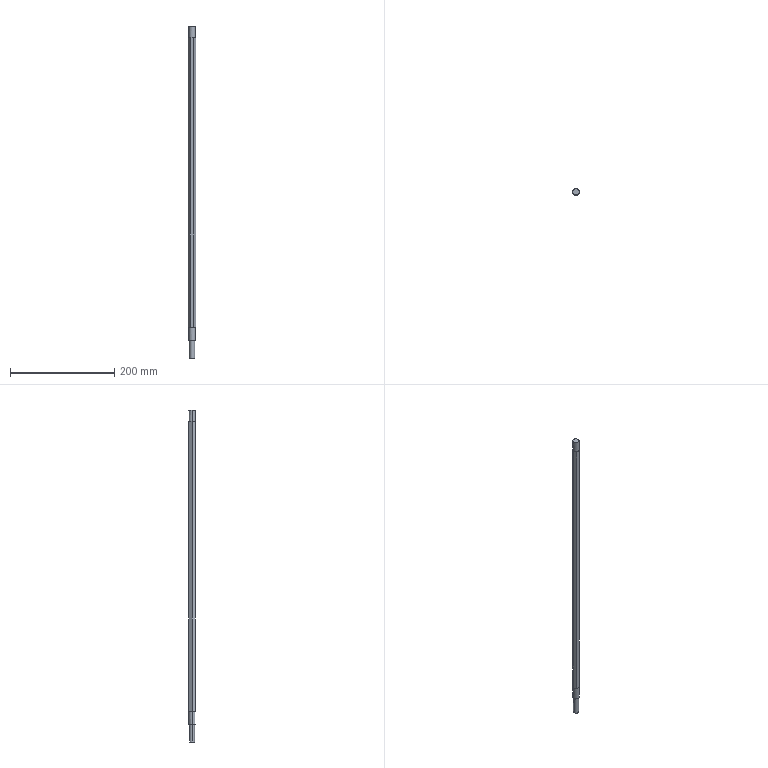Part | SolidWorks | features BaseBody 1 | 1 solid | 31 faces | box 13.856 x 12 x 637 mm | volume 77091 mm3 | plane 24 | cylinder 7 | commonest cylinder face diameters 12 x4 10 x2 3 x1
STEP:
#1=CARTESIAN_POINT('',(-5.,0.,34.));
#2=VERTEX_POINT('',#1);
#3=CARTESIAN_POINT('',(5.,0.,34.));
#4=VERTEX_POINT('',#3);
#5=CARTESIAN_POINT('',(0.,0.,34.));
#6=DIRECTION('',(0.,0.,-1.));
#7=DIRECTION('',(-1.,0.,0.));
#8=AXIS2_PLACEMENT_3D('',#5,#6,#7);
#9=CIRCLE('',#8,5.);
#10=EDGE_CURVE('',#2,#4,#9,.T.);
#11=ORIENTED_EDGE('',*,*,#10,.T.);
#12=CARTESIAN_POINT('',(5.,0.,0.));
#13=VERTEX_POINT('',#12);
#14=CARTESIAN_POINT('',(5.,0.,34.));
#15=DIRECTION('',(0.,0.,-1.));
#16=VECTOR('',#15,1000.);
#17=LINE('',#14,#16);
#18=EDGE_CURVE('',#4,#13,#17,.T.);
#19=ORIENTED_EDGE('',*,*,#18,.T.);
#20=CARTESIAN_POINT('',(1.5,4.77,0.));
#21=VERTEX_POINT('',#20);
#22=CARTESIAN_POINT('',(0.,0.,0.));
#23=DIRECTION('',(0.,0.,-1.));
#24=DIRECTION('',(-1.,0.,0.));
#25=AXIS2_PLACEMENT_3D('',#22,#23,#24);
#26=CIRCLE('',#25,5.);
#27=EDGE_CURVE('',#21,#13,#26,.T.);
#28=ORIENTED_EDGE('',*,*,#27,.F.);
#29=CARTESIAN_POINT('',(1.5,4.77,29.5));
#30=VERTEX_POINT('',#29);
#31=CARTESIAN_POINT('',(1.5,4.77,34.));
#32=DIRECTION('',(0.,0.,-1.));
#33=VECTOR('',#32,1000.);
#34=LINE('',#31,#33);
#35=EDGE_CURVE('',#30,#21,#34,.T.);
#36=ORIENTED_EDGE('',*,*,#35,.F.);
#37=CARTESIAN_POINT('',(-1.5,4.77,29.5));
#38=VERTEX_POINT('',#37);
#39=CARTESIAN_POINT('',(1.5,4.77,29.5));
#40=CARTESIAN_POINT('',(1.5,4.77,29.6));
#41=CARTESIAN_POINT('',(1.49,4.773,29.698));
#42=CARTESIAN_POINT('',(1.452,4.785,29.89));
#43=CARTESIAN_POINT('',(1.423,4.793,29.985));
#44=CARTESIAN_POINT('',(1.347,4.815,30.167));
#45=CARTESIAN_POINT('',(1.301,4.828,30.253));
#46=CARTESIAN_POINT('',(1.193,4.856,30.415));
#47=CARTESIAN_POINT('',(1.13,4.871,30.492));
#48=CARTESIAN_POINT('',(0.9236,4.916,30.698));
#49=CARTESIAN_POINT('',(0.7573,4.946,30.809));
#50=CARTESIAN_POINT('',(0.3971,4.988,30.96));
#51=CARTESIAN_POINT('',(0.1993,5.,31.));
#52=CARTESIAN_POINT('',(-0.09968,5.,31.));
#53=CARTESIAN_POINT('',(-0.1976,4.997,30.99));
#54=CARTESIAN_POINT('',(-0.39,4.986,30.952));
#55=CARTESIAN_POINT('',(-0.4855,4.977,30.923));
#56=CARTESIAN_POINT('',(-0.6668,4.956,30.847));
#57=CARTESIAN_POINT('',(-0.7527,4.944,30.801));
#58=CARTESIAN_POINT('',(-0.9153,4.916,30.692));
#59=CARTESIAN_POINT('',(-0.9918,4.901,30.63));
#60=CARTESIAN_POINT('',(-1.198,4.856,30.423));
#61=CARTESIAN_POINT('',(-1.309,4.826,30.257));
#62=CARTESIAN_POINT('',(-1.46,4.783,29.897));
#63=CARTESIAN_POINT('',(-1.5,4.77,29.699));
#64=CARTESIAN_POINT('',(-1.5,4.77,29.5));
#65=B_SPLINE_CURVE_WITH_KNOTS('',3,(#39,#40,#41,#42,#43,#44,#45,#46,#47,#48,#49,#50,#51,#52,#53,#54,#55,#56,#57,#58,#59,#60,#61,#62,#63,#64),.UNSPECIFIED.,.F.,.F.,(4,2,2,2,2,2,2,2,2,2,2,2,4),(0.,0.0002946,0.0005892,0.0008838,0.001178,0.001768,0.002357,0.002652,0.002946,0.003241,0.003535,0.004125,0.004714),.UNSPECIFIED.);
#66=EDGE_CURVE('',#30,#38,#65,.T.);
#67=ORIENTED_EDGE('',*,*,#66,.T.);
#68=CARTESIAN_POINT('',(-1.5,4.77,0.));
#69=VERTEX_POINT('',#68);
#70=CARTESIAN_POINT('',(-1.5,4.77,34.));
#71=DIRECTION('',(0.,0.,1.));
#72=VECTOR('',#71,1000.);
#73=LINE('',#70,#72);
#74=EDGE_CURVE('',#69,#38,#73,.T.);
#75=ORIENTED_EDGE('',*,*,#74,.F.);
#76=CARTESIAN_POINT('',(-5.,0.,0.));
#77=VERTEX_POINT('',#76);
#78=CARTESIAN_POINT('',(0.,0.,0.));
#79=DIRECTION('',(0.,0.,-1.));
#80=DIRECTION('',(-1.,0.,0.));
#81=AXIS2_PLACEMENT_3D('',#78,#79,#80);
#82=CIRCLE('',#81,5.);
#83=EDGE_CURVE('',#77,#69,#82,.T.);
#84=ORIENTED_EDGE('',*,*,#83,.F.);
#85=CARTESIAN_POINT('',(-5.,0.,34.));
#86=DIRECTION('',(0.,0.,-1.));
#87=VECTOR('',#86,1000.);
#88=LINE('',#85,#87);
#89=EDGE_CURVE('',#2,#77,#88,.T.);
#90=ORIENTED_EDGE('',*,*,#89,.F.);
#91=EDGE_LOOP('',(#11,#19,#28,#36,#67,#75,#84,#90));
#92=FACE_OUTER_BOUND('',#91,.T.);
#93=CARTESIAN_POINT('',(0.,0.,34.));
#94=DIRECTION('',(0.,0.,-1.));
#95=DIRECTION('',(-1.,0.,0.));
#96=AXIS2_PLACEMENT_3D('',#93,#94,#95);
#97=CYLINDRICAL_SURFACE('',#96,5.);
#98=ADVANCED_FACE('',(#92),#97,.T.);
#99=CARTESIAN_POINT('',(-5.196,3.,615.));
#100=VERTEX_POINT('',#99);
#101=CARTESIAN_POINT('',(-6.,0.,615.));
#102=VERTEX_POINT('',#101);
#103=CARTESIAN_POINT('',(0.,0.,615.));
#104=DIRECTION('',(0.,0.,1.));
#105=DIRECTION('',(1.,0.,0.));
#106=AXIS2_PLACEMENT_3D('',#103,#104,#105);
#107=CIRCLE('',#106,6.);
#108=EDGE_CURVE('',#100,#102,#107,.T.);
#109=ORIENTED_EDGE('',*,*,#108,.T.);
#110=CARTESIAN_POINT('',(-6.,0.,637.));
#111=VERTEX_POINT('',#110);
#112=CARTESIAN_POINT('',(-6.,0.,615.));
#113=DIRECTION('',(0.,0.,1.));
#114=VECTOR('',#113,1000.);
#115=LINE('',#112,#114);
#116=EDGE_CURVE('',#102,#111,#115,.T.);
#117=ORIENTED_EDGE('',*,*,#116,.T.);
#118=CARTESIAN_POINT('',(6.,0.,637.));
#119=VERTEX_POINT('',#118);
#120=CARTESIAN_POINT('',(0.,0.,637.));
#121=DIRECTION('',(0.,0.,1.));
#122=DIRECTION('',(1.,0.,0.));
#123=AXIS2_PLACEMENT_3D('',#120,#121,#122);
#124=CIRCLE('',#123,6.);
#125=EDGE_CURVE('',#119,#111,#124,.T.);
#126=ORIENTED_EDGE('',*,*,#125,.F.);
#127=CARTESIAN_POINT('',(6.,0.,615.));
#128=VERTEX_POINT('',#127);
#129=CARTESIAN_POINT('',(6.,0.,615.));
#130=DIRECTION('',(0.,0.,1.));
#131=VECTOR('',#130,1000.);
#132=LINE('',#129,#131);
#133=EDGE_CURVE('',#128,#119,#132,.T.);
#134=ORIENTED_EDGE('',*,*,#133,.F.);
#135=CARTESIAN_POINT('',(5.196,3.,615.));
#136=VERTEX_POINT('',#135);
#137=CARTESIAN_POINT('',(0.,0.,615.));
#138=DIRECTION('',(0.,0.,1.));
#139=DIRECTION('',(1.,0.,0.));
#140=AXIS2_PLACEMENT_3D('',#137,#138,#139);
#141=CIRCLE('',#140,6.);
#142=EDGE_CURVE('',#128,#136,#141,.T.);
#143=ORIENTED_EDGE('',*,*,#142,.T.);
#144=CARTESIAN_POINT('',(0.,6.,615.));
#145=VERTEX_POINT('',#144);
#146=CARTESIAN_POINT('',(0.,0.,615.));
#147=DIRECTION('',(0.,0.,1.));
#148=DIRECTION('',(1.,0.,0.));
#149=AXIS2_PLACEMENT_3D('',#146,#147,#148);
#150=CIRCLE('',#149,6.);
#151=EDGE_CURVE('',#136,#145,#150,.T.);
#152=ORIENTED_EDGE('',*,*,#151,.T.);
#153=CARTESIAN_POINT('',(0.,0.,615.));
#154=DIRECTION('',(0.,0.,1.));
#155=DIRECTION('',(1.,0.,0.));
#156=AXIS2_PLACEMENT_3D('',#153,#154,#155);
#157=CIRCLE('',#156,6.);
#158=EDGE_CURVE('',#145,#100,#157,.T.);
#159=ORIENTED_EDGE('',*,*,#158,.T.);
#160=EDGE_LOOP('',(#109,#117,#126,#134,#143,#152,#159));
#161=FACE_OUTER_BOUND('',#160,.T.);
#162=CARTESIAN_POINT('',(0.,0.,615.));
#163=DIRECTION('',(0.,0.,1.));
#164=DIRECTION('',(1.,0.,0.));
#165=AXIS2_PLACEMENT_3D('',#162,#163,#164);
#166=CYLINDRICAL_SURFACE('',#165,6.);
#167=ADVANCED_FACE('',(#161),#166,.T.);
#168=CARTESIAN_POINT('',(5.196,3.,59.));
#169=VERTEX_POINT('',#168);
#170=CARTESIAN_POINT('',(6.,0.,59.));
#171=VERTEX_POINT('',#170);
#172=CARTESIAN_POINT('',(0.,0.,59.));
#173=DIRECTION('',(0.,0.,-1.));
#174=DIRECTION('',(-1.,0.,0.));
#175=AXIS2_PLACEMENT_3D('',#172,#173,#174);
#176=CIRCLE('',#175,6.);
#177=EDGE_CURVE('',#169,#171,#176,.T.);
#178=ORIENTED_EDGE('',*,*,#177,.T.);
#179=CARTESIAN_POINT('',(6.,0.,34.));
#180=VERTEX_POINT('',#179);
#181=CARTESIAN_POINT('',(6.,0.,59.));
#182=DIRECTION('',(0.,0.,-1.));
#183=VECTOR('',#182,1000.);
#184=LINE('',#181,#183);
#185=EDGE_CURVE('',#171,#180,#184,.T.);
#186=ORIENTED_EDGE('',*,*,#185,.T.);
#187=CARTESIAN_POINT('',(-6.,0.,34.));
#188=VERTEX_POINT('',#187);
#189=CARTESIAN_POINT('',(0.,0.,34.));
#190=DIRECTION('',(0.,0.,1.));
#191=DIRECTION('',(-1.,0.,0.));
#192=AXIS2_PLACEMENT_3D('',#189,#190,#191);
#193=CIRCLE('',#192,6.);
#194=EDGE_CURVE('',#180,#188,#193,.T.);
#195=ORIENTED_EDGE('',*,*,#194,.T.);
#196=CARTESIAN_POINT('',(-6.,0.,59.));
#197=VERTEX_POINT('',#196);
#198=CARTESIAN_POINT('',(-6.,0.,59.));
#199=DIRECTION('',(0.,0.,-1.));
#200=VECTOR('',#199,1000.);
#201=LINE('',#198,#200);
#202=EDGE_CURVE('',#197,#188,#201,.T.);
#203=ORIENTED_EDGE('',*,*,#202,.F.);
#204=CARTESIAN_POINT('',(-5.196,3.,59.));
#205=VERTEX_POINT('',#204);
#206=CARTESIAN_POINT('',(0.,0.,59.));
#207=DIRECTION('',(0.,0.,-1.));
#208=DIRECTION('',(-1.,0.,0.));
#209=AXIS2_PLACEMENT_3D('',#206,#207,#208);
#210=CIRCLE('',#209,6.);
#211=EDGE_CURVE('',#197,#205,#210,.T.);
#212=ORIENTED_EDGE('',*,*,#211,.T.);
#213=CARTESIAN_POINT('',(0.,6.,59.));
#214=VERTEX_POINT('',#213);
#215=CARTESIAN_POINT('',(0.,0.,59.));
#216=DIRECTION('',(0.,0.,-1.));
#217=DIRECTION('',(-1.,0.,0.));
#218=AXIS2_PLACEMENT_3D('',#215,#216,#217);
#219=CIRCLE('',#218,6.);
#220=EDGE_CURVE('',#205,#214,#219,.T.);
#221=ORIENTED_EDGE('',*,*,#220,.T.);
#222=CARTESIAN_POINT('',(0.,0.,59.));
#223=DIRECTION('',(0.,0.,-1.));
#224=DIRECTION('',(-1.,0.,0.));
#225=AXIS2_PLACEMENT_3D('',#222,#223,#224);
#226=CIRCLE('',#225,6.);
#227=EDGE_CURVE('',#214,#169,#226,.T.);
#228=ORIENTED_EDGE('',*,*,#227,.T.);
#229=EDGE_LOOP('',(#178,#186,#195,#203,#212,#221,#228));
#230=FACE_OUTER_BOUND('',#229,.T.);
#231=CARTESIAN_POINT('',(0.,0.,59.));
#232=DIRECTION('',(0.,0.,-1.));
#233=DIRECTION('',(-1.,0.,0.));
#234=AXIS2_PLACEMENT_3D('',#231,#232,#233);
#235=CYLINDRICAL_SURFACE('',#234,6.);
#236=ADVANCED_FACE('',(#230),#235,.T.);
#237=CARTESIAN_POINT('',(1.5,2.398,29.5));
#238=VERTEX_POINT('',#237);
#239=CARTESIAN_POINT('',(1.5,7.398,29.5));
#240=DIRECTION('',(0.,1.,0.));
#241=VECTOR('',#240,1000.);
#242=LINE('',#239,#241);
#243=EDGE_CURVE('',#238,#30,#242,.T.);
#244=ORIENTED_EDGE('',*,*,#243,.F.);
#245=CARTESIAN_POINT('',(-1.5,2.398,29.5));
#246=VERTEX_POINT('',#245);
#247=CARTESIAN_POINT('',(0.,2.398,29.5));
#248=DIRECTION('',(0.,1.,0.));
#249=DIRECTION('',(1.,0.,0.));
#250=AXIS2_PLACEMENT_3D('',#247,#248,#249);
#251=CIRCLE('',#250,1.5);
#252=EDGE_CURVE('',#246,#238,#251,.T.);
#253=ORIENTED_EDGE('',*,*,#252,.F.);
#254=CARTESIAN_POINT('',(-1.5,7.398,29.5));
#255=DIRECTION('',(0.,-1.,0.));
#256=VECTOR('',#255,1000.);
#257=LINE('',#254,#256);
#258=EDGE_CURVE('',#38,#246,#257,.T.);
#259=ORIENTED_EDGE('',*,*,#258,.F.);
#260=ORIENTED_EDGE('',*,*,#66,.F.);
#261=EDGE_LOOP('',(#244,#253,#259,#260));
#262=FACE_OUTER_BOUND('',#261,.T.);
#263=CARTESIAN_POINT('',(0.,0.,29.5));
#264=DIRECTION('',(0.,-1.,0.));
#265=DIRECTION('',(1.,0.,0.));
#266=AXIS2_PLACEMENT_3D('',#263,#264,#265);
#267=CYLINDRICAL_SURFACE('',#266,1.5);
#268=ADVANCED_FACE('',(#262),#267,.F.);
#269=CARTESIAN_POINT('',(-1.5,2.398,0.));
#270=VERTEX_POINT('',#269);
#271=CARTESIAN_POINT('',(-1.5,2.398,31.));
#272=DIRECTION('',(0.,0.,-1.));
#273=VECTOR('',#272,1000.);
#274=LINE('',#271,#273);
#275=EDGE_CURVE('',#246,#270,#274,.T.);
#276=ORIENTED_EDGE('',*,*,#275,.F.);
#277=ORIENTED_EDGE('',*,*,#252,.T.);
#278=CARTESIAN_POINT('',(1.5,2.398,0.));
#279=VERTEX_POINT('',#278);
#280=CARTESIAN_POINT('',(1.5,2.398,31.));
#281=DIRECTION('',(0.,0.,-1.));
#282=VECTOR('',#281,1000.);
#283=LINE('',#280,#282);
#284=EDGE_CURVE('',#238,#279,#283,.T.);
#285=ORIENTED_EDGE('',*,*,#284,.T.);
#286=CARTESIAN_POINT('',(1.5,2.398,0.));
#287=DIRECTION('',(-1.,0.,0.));
#288=VECTOR('',#287,1000.);
#289=LINE('',#286,#288);
#290=EDGE_CURVE('',#279,#270,#289,.T.);
#291=ORIENTED_EDGE('',*,*,#290,.T.);
#292=EDGE_LOOP('',(#276,#277,#285,#291));
#293=FACE_OUTER_BOUND('',#292,.T.);
#294=CARTESIAN_POINT('',(1.5,2.398,31.));
#295=DIRECTION('',(0.,-1.,0.));
#296=DIRECTION('',(-1.,0.,0.));
#297=AXIS2_PLACEMENT_3D('',#294,#295,#296);
#298=PLANE('',#297);
#299=ADVANCED_FACE('',(#293),#298,.F.);
#300=ORIENTED_EDGE('',*,*,#74,.T.);
#301=ORIENTED_EDGE('',*,*,#258,.T.);
#302=ORIENTED_EDGE('',*,*,#275,.T.);
#303=CARTESIAN_POINT('',(-1.5,7.398,0.));
#304=DIRECTION('',(0.,1.,0.));
#305=VECTOR('',#304,1000.);
#306=LINE('',#303,#305);
#307=EDGE_CURVE('',#270,#69,#306,.T.);
#308=ORIENTED_EDGE('',*,*,#307,.T.);
#309=EDGE_LOOP('',(#300,#301,#302,#308));
#310=FACE_OUTER_BOUND('',#309,.T.);
#311=CARTESIAN_POINT('',(-1.5,7.398,31.));
#312=DIRECTION('',(-1.,0.,0.));
#313=DIRECTION('',(0.,0.,1.));
#314=AXIS2_PLACEMENT_3D('',#311,#312,#313);
#315=PLANE('',#314);
#316=ADVANCED_FACE('',(#310),#315,.F.);
#317=ORIENTED_EDGE('',*,*,#284,.F.);
#318=ORIENTED_EDGE('',*,*,#243,.T.);
#319=ORIENTED_EDGE('',*,*,#35,.T.);
#320=CARTESIAN_POINT('',(1.5,0.,0.));
#321=DIRECTION('',(0.,1.,0.));
#322=VECTOR('',#321,1000.);
#323=LINE('',#320,#322);
#324=EDGE_CURVE('',#279,#21,#323,.T.);
#325=ORIENTED_EDGE('',*,*,#324,.F.);
#326=EDGE_LOOP('',(#317,#318,#319,#325));
#327=FACE_OUTER_BOUND('',#326,.T.);
#328=CARTESIAN_POINT('',(1.5,7.398,31.));
#329=DIRECTION('',(1.,0.,0.));
#330=DIRECTION('',(0.,1.,0.));
#331=AXIS2_PLACEMENT_3D('',#328,#329,#330);
#332=PLANE('',#331);
#333=ADVANCED_FACE('',(#327),#332,.F.);
#334=ORIENTED_EDGE('',*,*,#290,.F.);
#335=ORIENTED_EDGE('',*,*,#324,.T.);
#336=ORIENTED_EDGE('',*,*,#27,.T.);
#337=CARTESIAN_POINT('',(0.,0.,0.));
#338=DIRECTION('',(0.,0.,-1.));
#339=DIRECTION('',(-1.,0.,0.));
#340=AXIS2_PLACEMENT_3D('',#337,#338,#339);
#341=CIRCLE('',#340,5.);
#342=EDGE_CURVE('',#13,#77,#341,.T.);
#343=ORIENTED_EDGE('',*,*,#342,.T.);
#344=ORIENTED_EDGE('',*,*,#83,.T.);
#345=ORIENTED_EDGE('',*,*,#307,.F.);
#346=EDGE_LOOP('',(#334,#335,#336,#343,#344,#345));
#347=FACE_OUTER_BOUND('',#346,.T.);
#348=CARTESIAN_POINT('',(0.,0.,0.));
#349=DIRECTION('',(0.,0.,1.));
#350=DIRECTION('',(1.,0.,0.));
#351=AXIS2_PLACEMENT_3D('',#348,#349,#350);
#352=PLANE('',#351);
#353=ADVANCED_FACE('',(#347),#352,.F.);
#354=ORIENTED_EDGE('',*,*,#10,.F.);
#355=CARTESIAN_POINT('',(0.,0.,34.));
#356=DIRECTION('',(0.,0.,-1.));
#357=DIRECTION('',(-1.,0.,0.));
#358=AXIS2_PLACEMENT_3D('',#355,#356,#357);
#359=CIRCLE('',#358,5.);
#360=EDGE_CURVE('',#4,#2,#359,.T.);
#361=ORIENTED_EDGE('',*,*,#360,.F.);
#362=EDGE_LOOP('',(#354,#361));
#363=FACE_BOUND('',#362,.T.);
#364=CARTESIAN_POINT('',(0.,0.,34.));
#365=DIRECTION('',(0.,0.,1.));
#366=DIRECTION('',(-1.,0.,0.));
#367=AXIS2_PLACEMENT_3D('',#364,#365,#366);
#368=CIRCLE('',#367,6.);
#369=EDGE_CURVE('',#188,#180,#368,.T.);
#370=ORIENTED_EDGE('',*,*,#369,.F.);
#371=ORIENTED_EDGE('',*,*,#194,.F.);
#372=EDGE_LOOP('',(#370,#371));
#373=FACE_OUTER_BOUND('',#372,.T.);
#374=CARTESIAN_POINT('',(0.,0.,34.));
#375=DIRECTION('',(0.,0.,-1.));
#376=DIRECTION('',(0.,-1.,0.));
#377=AXIS2_PLACEMENT_3D('',#374,#375,#376);
#378=PLANE('',#377);
#379=ADVANCED_FACE('',(#363,#373),#378,.T.);
#380=CARTESIAN_POINT('',(-3.464,-6.,59.));
#381=VERTEX_POINT('',#380);
#382=CARTESIAN_POINT('',(-5.196,-3.,59.));
#383=VERTEX_POINT('',#382);
#384=CARTESIAN_POINT('',(-6.928,0.,59.));
#385=DIRECTION('',(-0.5,0.866,0.));
#386=VECTOR('',#385,1000.);
#387=LINE('',#384,#386);
#388=EDGE_CURVE('',#381,#383,#387,.T.);
#389=ORIENTED_EDGE('',*,*,#388,.T.);
#390=CARTESIAN_POINT('',(0.,-6.,59.));
#391=VERTEX_POINT('',#390);
#392=CARTESIAN_POINT('',(0.,0.,59.));
#393=DIRECTION('',(0.,0.,-1.));
#394=DIRECTION('',(-1.,0.,0.));
#395=AXIS2_PLACEMENT_3D('',#392,#393,#394);
#396=CIRCLE('',#395,6.);
#397=EDGE_CURVE('',#391,#383,#396,.T.);
#398=ORIENTED_EDGE('',*,*,#397,.F.);
#399=CARTESIAN_POINT('',(-3.464,-6.,59.));
#400=DIRECTION('',(-1.,0.,0.));
#401=VECTOR('',#400,1000.);
#402=LINE('',#399,#401);
#403=EDGE_CURVE('',#391,#381,#402,.T.);
#404=ORIENTED_EDGE('',*,*,#403,.T.);
#405=EDGE_LOOP('',(#389,#398,#404));
#406=FACE_OUTER_BOUND('',#405,.T.);
#407=CARTESIAN_POINT('',(0.,0.,59.));
#408=DIRECTION('',(0.,0.,-1.));
#409=DIRECTION('',(0.,-1.,0.));
#410=AXIS2_PLACEMENT_3D('',#407,#408,#409);
#411=PLANE('',#410);
#412=ADVANCED_FACE('',(#406),#411,.T.);
#413=CARTESIAN_POINT('',(5.196,-3.,59.));
#414=VERTEX_POINT('',#413);
#415=CARTESIAN_POINT('',(3.464,-6.,59.));
#416=VERTEX_POINT('',#415);
#417=CARTESIAN_POINT('',(3.464,-6.,59.));
#418=DIRECTION('',(-0.5,-0.866,0.));
#419=VECTOR('',#418,1000.);
#420=LINE('',#417,#419);
#421=EDGE_CURVE('',#414,#416,#420,.T.);
#422=ORIENTED_EDGE('',*,*,#421,.T.);
#423=CARTESIAN_POINT('',(-3.464,-6.,59.));
#424=DIRECTION('',(-1.,0.,0.));
#425=VECTOR('',#424,1000.);
#426=LINE('',#423,#425);
#427=EDGE_CURVE('',#416,#391,#426,.T.);
#428=ORIENTED_EDGE('',*,*,#427,.T.);
#429=CARTESIAN_POINT('',(0.,0.,59.));
#430=DIRECTION('',(0.,0.,-1.));
#431=DIRECTION('',(-1.,0.,0.));
#432=AXIS2_PLACEMENT_3D('',#429,#430,#431);
#433=CIRCLE('',#432,6.);
#434=EDGE_CURVE('',#414,#391,#433,.T.);
#435=ORIENTED_EDGE('',*,*,#434,.F.);
#436=EDGE_LOOP('',(#422,#428,#435));
#437=FACE_OUTER_BOUND('',#436,.T.);
#438=CARTESIAN_POINT('',(0.,0.,59.));
#439=DIRECTION('',(0.,0.,-1.));
#440=DIRECTION('',(0.,-1.,0.));
#441=AXIS2_PLACEMENT_3D('',#438,#439,#440);
#442=PLANE('',#441);
#443=ADVANCED_FACE('',(#437),#442,.T.);
#444=CARTESIAN_POINT('',(-6.928,0.,59.));
#445=VERTEX_POINT('',#444);
#446=CARTESIAN_POINT('',(-3.464,6.,59.));
#447=DIRECTION('',(0.5,0.866,0.));
#448=VECTOR('',#447,1000.);
#449=LINE('',#446,#448);
#450=EDGE_CURVE('',#445,#205,#449,.T.);
#451=ORIENTED_EDGE('',*,*,#450,.T.);
#452=ORIENTED_EDGE('',*,*,#211,.F.);
#453=CARTESIAN_POINT('',(0.,0.,59.));
#454=DIRECTION('',(0.,0.,-1.));
#455=DIRECTION('',(-1.,0.,0.));
#456=AXIS2_PLACEMENT_3D('',#453,#454,#455);
#457=CIRCLE('',#456,6.);
#458=EDGE_CURVE('',#383,#197,#457,.T.);
#459=ORIENTED_EDGE('',*,*,#458,.F.);
#460=CARTESIAN_POINT('',(-6.928,0.,59.));
#461=DIRECTION('',(-0.5,0.866,0.));
#462=VECTOR('',#461,1000.);
#463=LINE('',#460,#462);
#464=EDGE_CURVE('',#383,#445,#463,.T.);
#465=ORIENTED_EDGE('',*,*,#464,.T.);
#466=EDGE_LOOP('',(#451,#452,#459,#465));
#467=FACE_OUTER_BOUND('',#466,.T.);
#468=CARTESIAN_POINT('',(0.,0.,59.));
#469=DIRECTION('',(0.,0.,-1.));
#470=DIRECTION('',(0.,-1.,0.));
#471=AXIS2_PLACEMENT_3D('',#468,#469,#470);
#472=PLANE('',#471);
#473=ADVANCED_FACE('',(#467),#472,.T.);
#474=CARTESIAN_POINT('',(6.928,0.,59.));
#475=VERTEX_POINT('',#474);
#476=CARTESIAN_POINT('',(6.928,0.,59.));
#477=DIRECTION('',(0.5,-0.866,0.));
#478=VECTOR('',#477,1000.);
#479=LINE('',#476,#478);
#480=EDGE_CURVE('',#169,#475,#479,.T.);
#481=ORIENTED_EDGE('',*,*,#480,.T.);
#482=CARTESIAN_POINT('',(3.464,-6.,59.));
#483=DIRECTION('',(-0.5,-0.866,0.));
#484=VECTOR('',#483,1000.);
#485=LINE('',#482,#484);
#486=EDGE_CURVE('',#475,#414,#485,.T.);
#487=ORIENTED_EDGE('',*,*,#486,.T.);
#488=CARTESIAN_POINT('',(0.,0.,59.));
#489=DIRECTION('',(0.,0.,-1.));
#490=DIRECTION('',(-1.,0.,0.));
#491=AXIS2_PLACEMENT_3D('',#488,#489,#490);
#492=CIRCLE('',#491,6.);
#493=EDGE_CURVE('',#171,#414,#492,.T.);
#494=ORIENTED_EDGE('',*,*,#493,.F.);
#495=ORIENTED_EDGE('',*,*,#177,.F.);
#496=EDGE_LOOP('',(#481,#487,#494,#495));
#497=FACE_OUTER_BOUND('',#496,.T.);
#498=CARTESIAN_POINT('',(0.,0.,59.));
#499=DIRECTION('',(0.,0.,-1.));
#500=DIRECTION('',(0.,-1.,0.));
#501=AXIS2_PLACEMENT_3D('',#498,#499,#500);
#502=PLANE('',#501);
#503=ADVANCED_FACE('',(#497),#502,.T.);
#504=CARTESIAN_POINT('',(3.464,6.,59.));
#505=VERTEX_POINT('',#504);
#506=CARTESIAN_POINT('',(3.464,6.,59.));
#507=DIRECTION('',(1.,0.,0.));
#508=VECTOR('',#507,1000.);
#509=LINE('',#506,#508);
#510=EDGE_CURVE('',#214,#505,#509,.T.);
#511=ORIENTED_EDGE('',*,*,#510,.T.);
#512=CARTESIAN_POINT('',(6.928,0.,59.));
#513=DIRECTION('',(0.5,-0.866,0.));
#514=VECTOR('',#513,1000.);
#515=LINE('',#512,#514);
#516=EDGE_CURVE('',#505,#169,#515,.T.);
#517=ORIENTED_EDGE('',*,*,#516,.T.);
#518=ORIENTED_EDGE('',*,*,#227,.F.);
#519=EDGE_LOOP('',(#511,#517,#518));
#520=FACE_OUTER_BOUND('',#519,.T.);
#521=CARTESIAN_POINT('',(0.,0.,59.));
#522=DIRECTION('',(0.,0.,-1.));
#523=DIRECTION('',(0.,-1.,0.));
#524=AXIS2_PLACEMENT_3D('',#521,#522,#523);
#525=PLANE('',#524);
#526=ADVANCED_FACE('',(#520),#525,.T.);
#527=CARTESIAN_POINT('',(-3.464,6.,59.));
#528=VERTEX_POINT('',#527);
#529=CARTESIAN_POINT('',(3.464,6.,59.));
#530=DIRECTION('',(1.,0.,0.));
#531=VECTOR('',#530,1000.);
#532=LINE('',#529,#531);
#533=EDGE_CURVE('',#528,#214,#532,.T.);
#534=ORIENTED_EDGE('',*,*,#533,.T.);
#535=ORIENTED_EDGE('',*,*,#220,.F.);
#536=CARTESIAN_POINT('',(-3.464,6.,59.));
#537=DIRECTION('',(0.5,0.866,0.));
#538=VECTOR('',#537,1000.);
#539=LINE('',#536,#538);
#540=EDGE_CURVE('',#205,#528,#539,.T.);
#541=ORIENTED_EDGE('',*,*,#540,.T.);
#542=EDGE_LOOP('',(#534,#535,#541));
#543=FACE_OUTER_BOUND('',#542,.T.);
#544=CARTESIAN_POINT('',(0.,0.,59.));
#545=DIRECTION('',(0.,0.,-1.));
#546=DIRECTION('',(0.,-1.,0.));
#547=AXIS2_PLACEMENT_3D('',#544,#545,#546);
#548=PLANE('',#547);
#549=ADVANCED_FACE('',(#543),#548,.T.);
#550=ORIENTED_EDGE('',*,*,#125,.T.);
#551=CARTESIAN_POINT('',(0.,0.,637.));
#552=DIRECTION('',(0.,0.,1.));
#553=DIRECTION('',(1.,0.,0.));
#554=AXIS2_PLACEMENT_3D('',#551,#552,#553);
#555=CIRCLE('',#554,6.);
#556=EDGE_CURVE('',#111,#119,#555,.T.);
#557=ORIENTED_EDGE('',*,*,#556,.T.);
#558=EDGE_LOOP('',(#550,#557));
#559=FACE_OUTER_BOUND('',#558,.T.);
#560=CARTESIAN_POINT('',(0.,0.,637.));
#561=DIRECTION('',(0.,0.,1.));
#562=DIRECTION('',(1.,0.,0.));
#563=AXIS2_PLACEMENT_3D('',#560,#561,#562);
#564=PLANE('',#563);
#565=ADVANCED_FACE('',(#559),#564,.T.);
#566=CARTESIAN_POINT('',(-5.196,-3.,615.));
#567=VERTEX_POINT('',#566);
#568=CARTESIAN_POINT('',(-3.464,-6.,615.));
#569=VERTEX_POINT('',#568);
#570=CARTESIAN_POINT('',(-6.928,0.,615.));
#571=DIRECTION('',(0.5,-0.866,0.));
#572=VECTOR('',#571,1000.);
#573=LINE('',#570,#572);
#574=EDGE_CURVE('',#567,#569,#573,.T.);
#575=ORIENTED_EDGE('',*,*,#574,.T.);
#576=CARTESIAN_POINT('',(0.,-6.,615.));
#577=VERTEX_POINT('',#576);
#578=CARTESIAN_POINT('',(-3.464,-6.,615.));
#579=DIRECTION('',(1.,0.,0.));
#580=VECTOR('',#579,1000.);
#581=LINE('',#578,#580);
#582=EDGE_CURVE('',#569,#577,#581,.T.);
#583=ORIENTED_EDGE('',*,*,#582,.T.);
#584=CARTESIAN_POINT('',(0.,0.,615.));
#585=DIRECTION('',(0.,0.,1.));
#586=DIRECTION('',(1.,0.,0.));
#587=AXIS2_PLACEMENT_3D('',#584,#585,#586);
#588=CIRCLE('',#587,6.);
#589=EDGE_CURVE('',#567,#577,#588,.T.);
#590=ORIENTED_EDGE('',*,*,#589,.F.);
#591=EDGE_LOOP('',(#575,#583,#590));
#592=FACE_OUTER_BOUND('',#591,.T.);
#593=CARTESIAN_POINT('',(0.,0.,615.));
#594=DIRECTION('',(0.,0.,1.));
#595=DIRECTION('',(1.,0.,0.));
#596=AXIS2_PLACEMENT_3D('',#593,#594,#595);
#597=PLANE('',#596);
#598=ADVANCED_FACE('',(#592),#597,.T.);
#599=CARTESIAN_POINT('',(-6.928,0.,615.));
#600=VERTEX_POINT('',#599);
#601=CARTESIAN_POINT('',(-3.464,6.,615.));
#602=DIRECTION('',(-0.5,-0.866,0.));
#603=VECTOR('',#602,1000.);
#604=LINE('',#601,#603);
#605=EDGE_CURVE('',#100,#600,#604,.T.);
#606=ORIENTED_EDGE('',*,*,#605,.T.);
#607=CARTESIAN_POINT('',(-6.928,0.,615.));
#608=DIRECTION('',(0.5,-0.866,0.));
#609=VECTOR('',#608,1000.);
#610=LINE('',#607,#609);
#611=EDGE_CURVE('',#600,#567,#610,.T.);
#612=ORIENTED_EDGE('',*,*,#611,.T.);
#613=CARTESIAN_POINT('',(0.,0.,615.));
#614=DIRECTION('',(0.,0.,1.));
#615=DIRECTION('',(1.,0.,0.));
#616=AXIS2_PLACEMENT_3D('',#613,#614,#615);
#617=CIRCLE('',#616,6.);
#618=EDGE_CURVE('',#102,#567,#617,.T.);
#619=ORIENTED_EDGE('',*,*,#618,.F.);
#620=ORIENTED_EDGE('',*,*,#108,.F.);
#621=EDGE_LOOP('',(#606,#612,#619,#620));
#622=FACE_OUTER_BOUND('',#621,.T.);
#623=CARTESIAN_POINT('',(0.,0.,615.));
#624=DIRECTION('',(0.,0.,1.));
#625=DIRECTION('',(1.,0.,0.));
#626=AXIS2_PLACEMENT_3D('',#623,#624,#625);
#627=PLANE('',#626);
#628=ADVANCED_FACE('',(#622),#627,.T.);
#629=CARTESIAN_POINT('',(-3.464,6.,615.));
#630=VERTEX_POINT('',#629);
#631=CARTESIAN_POINT('',(3.464,6.,615.));
#632=DIRECTION('',(-1.,0.,0.));
#633=VECTOR('',#632,1000.);
#634=LINE('',#631,#633);
#635=EDGE_CURVE('',#145,#630,#634,.T.);
#636=ORIENTED_EDGE('',*,*,#635,.T.);
#637=CARTESIAN_POINT('',(-3.464,6.,615.));
#638=DIRECTION('',(-0.5,-0.866,0.));
#639=VECTOR('',#638,1000.);
#640=LINE('',#637,#639);
#641=EDGE_CURVE('',#630,#100,#640,.T.);
#642=ORIENTED_EDGE('',*,*,#641,.T.);
#643=ORIENTED_EDGE('',*,*,#158,.F.);
#644=EDGE_LOOP('',(#636,#642,#643));
#645=FACE_OUTER_BOUND('',#644,.T.);
#646=CARTESIAN_POINT('',(0.,0.,615.));
#647=DIRECTION('',(0.,0.,1.));
#648=DIRECTION('',(1.,0.,0.));
#649=AXIS2_PLACEMENT_3D('',#646,#647,#648);
#650=PLANE('',#649);
#651=ADVANCED_FACE('',(#645),#650,.T.);
#652=CARTESIAN_POINT('',(3.464,6.,615.));
#653=VERTEX_POINT('',#652);
#654=CARTESIAN_POINT('',(6.928,0.,615.));
#655=DIRECTION('',(-0.5,0.866,0.));
#656=VECTOR('',#655,1000.);
#657=LINE('',#654,#656);
#658=EDGE_CURVE('',#136,#653,#657,.T.);
#659=ORIENTED_EDGE('',*,*,#658,.T.);
#660=CARTESIAN_POINT('',(3.464,6.,615.));
#661=DIRECTION('',(-1.,0.,0.));
#662=VECTOR('',#661,1000.);
#663=LINE('',#660,#662);
#664=EDGE_CURVE('',#653,#145,#663,.T.);
#665=ORIENTED_EDGE('',*,*,#664,.T.);
#666=ORIENTED_EDGE('',*,*,#151,.F.);
#667=EDGE_LOOP('',(#659,#665,#666));
#668=FACE_OUTER_BOUND('',#667,.T.);
#669=CARTESIAN_POINT('',(0.,0.,615.));
#670=DIRECTION('',(0.,0.,1.));
#671=DIRECTION('',(1.,0.,0.));
#672=AXIS2_PLACEMENT_3D('',#669,#670,#671);
#673=PLANE('',#672);
#674=ADVANCED_FACE('',(#668),#673,.T.);
#675=CARTESIAN_POINT('',(5.196,-3.,615.));
#676=VERTEX_POINT('',#675);
#677=CARTESIAN_POINT('',(6.928,0.,615.));
#678=VERTEX_POINT('',#677);
#679=CARTESIAN_POINT('',(3.464,-6.,615.));
#680=DIRECTION('',(0.5,0.866,0.));
#681=VECTOR('',#680,1000.);
#682=LINE('',#679,#681);
#683=EDGE_CURVE('',#676,#678,#682,.T.);
#684=ORIENTED_EDGE('',*,*,#683,.T.);
#685=CARTESIAN_POINT('',(6.928,0.,615.));
#686=DIRECTION('',(-0.5,0.866,0.));
#687=VECTOR('',#686,1000.);
#688=LINE('',#685,#687);
#689=EDGE_CURVE('',#678,#136,#688,.T.);
#690=ORIENTED_EDGE('',*,*,#689,.T.);
#691=ORIENTED_EDGE('',*,*,#142,.F.);
#692=CARTESIAN_POINT('',(0.,0.,615.));
#693=DIRECTION('',(0.,0.,1.));
#694=DIRECTION('',(1.,0.,0.));
#695=AXIS2_PLACEMENT_3D('',#692,#693,#694);
#696=CIRCLE('',#695,6.);
#697=EDGE_CURVE('',#676,#128,#696,.T.);
#698=ORIENTED_EDGE('',*,*,#697,.F.);
#699=EDGE_LOOP('',(#684,#690,#691,#698));
#700=FACE_OUTER_BOUND('',#699,.T.);
#701=CARTESIAN_POINT('',(0.,0.,615.));
#702=DIRECTION('',(0.,0.,1.));
#703=DIRECTION('',(1.,0.,0.));
#704=AXIS2_PLACEMENT_3D('',#701,#702,#703);
#705=PLANE('',#704);
#706=ADVANCED_FACE('',(#700),#705,.T.);
#707=CARTESIAN_POINT('',(3.464,-6.,615.));
#708=VERTEX_POINT('',#707);
#709=CARTESIAN_POINT('',(3.464,-6.,615.));
#710=DIRECTION('',(0.5,0.866,0.));
#711=VECTOR('',#710,1000.);
#712=LINE('',#709,#711);
#713=EDGE_CURVE('',#708,#676,#712,.T.);
#714=ORIENTED_EDGE('',*,*,#713,.T.);
#715=CARTESIAN_POINT('',(0.,0.,615.));
#716=DIRECTION('',(0.,0.,1.));
#717=DIRECTION('',(1.,0.,0.));
#718=AXIS2_PLACEMENT_3D('',#715,#716,#717);
#719=CIRCLE('',#718,6.);
#720=EDGE_CURVE('',#577,#676,#719,.T.);
#721=ORIENTED_EDGE('',*,*,#720,.F.);
#722=CARTESIAN_POINT('',(-3.464,-6.,615.));
#723=DIRECTION('',(1.,0.,0.));
#724=VECTOR('',#723,1000.);
#725=LINE('',#722,#724);
#726=EDGE_CURVE('',#577,#708,#725,.T.);
#727=ORIENTED_EDGE('',*,*,#726,.T.);
#728=EDGE_LOOP('',(#714,#721,#727));
#729=FACE_OUTER_BOUND('',#728,.T.);
#730=CARTESIAN_POINT('',(0.,0.,615.));
#731=DIRECTION('',(0.,0.,1.));
#732=DIRECTION('',(1.,0.,0.));
#733=AXIS2_PLACEMENT_3D('',#730,#731,#732);
#734=PLANE('',#733);
#735=ADVANCED_FACE('',(#729),#734,.T.);
#736=ORIENTED_EDGE('',*,*,#427,.F.);
#737=CARTESIAN_POINT('',(3.464,-6.,637.));
#738=DIRECTION('',(0.,0.,-1.));
#739=VECTOR('',#738,1000.);
#740=LINE('',#737,#739);
#741=EDGE_CURVE('',#708,#416,#740,.T.);
#742=ORIENTED_EDGE('',*,*,#741,.F.);
#743=ORIENTED_EDGE('',*,*,#726,.F.);
#744=ORIENTED_EDGE('',*,*,#582,.F.);
#745=CARTESIAN_POINT('',(-3.464,-6.,637.));
#746=DIRECTION('',(0.,0.,-1.));
#747=VECTOR('',#746,1000.);
#748=LINE('',#745,#747);
#749=EDGE_CURVE('',#569,#381,#748,.T.);
#750=ORIENTED_EDGE('',*,*,#749,.T.);
#751=ORIENTED_EDGE('',*,*,#403,.F.);
#752=EDGE_LOOP('',(#736,#742,#743,#744,#750,#751));
#753=FACE_OUTER_BOUND('',#752,.T.);
#754=CARTESIAN_POINT('',(-3.464,-6.,637.));
#755=DIRECTION('',(0.,1.,0.));
#756=DIRECTION('',(1.,0.,0.));
#757=AXIS2_PLACEMENT_3D('',#754,#755,#756);
#758=PLANE('',#757);
#759=ADVANCED_FACE('',(#753),#758,.F.);
#760=ORIENTED_EDGE('',*,*,#388,.F.);
#761=ORIENTED_EDGE('',*,*,#749,.F.);
#762=ORIENTED_EDGE('',*,*,#574,.F.);
#763=ORIENTED_EDGE('',*,*,#611,.F.);
#764=CARTESIAN_POINT('',(-6.928,0.,637.));
#765=DIRECTION('',(0.,0.,-1.));
#766=VECTOR('',#765,1000.);
#767=LINE('',#764,#766);
#768=EDGE_CURVE('',#600,#445,#767,.T.);
#769=ORIENTED_EDGE('',*,*,#768,.T.);
#770=ORIENTED_EDGE('',*,*,#464,.F.);
#771=EDGE_LOOP('',(#760,#761,#762,#763,#769,#770));
#772=FACE_OUTER_BOUND('',#771,.T.);
#773=CARTESIAN_POINT('',(-6.928,0.,637.));
#774=DIRECTION('',(0.866,0.5,0.));
#775=DIRECTION('',(0.,0.,-1.));
#776=AXIS2_PLACEMENT_3D('',#773,#774,#775);
#777=PLANE('',#776);
#778=ADVANCED_FACE('',(#772),#777,.F.);
#779=ORIENTED_EDGE('',*,*,#450,.F.);
#780=ORIENTED_EDGE('',*,*,#768,.F.);
#781=ORIENTED_EDGE('',*,*,#605,.F.);
#782=ORIENTED_EDGE('',*,*,#641,.F.);
#783=CARTESIAN_POINT('',(-3.464,6.,637.));
#784=DIRECTION('',(0.,0.,-1.));
#785=VECTOR('',#784,1000.);
#786=LINE('',#783,#785);
#787=EDGE_CURVE('',#630,#528,#786,.T.);
#788=ORIENTED_EDGE('',*,*,#787,.T.);
#789=ORIENTED_EDGE('',*,*,#540,.F.);
#790=EDGE_LOOP('',(#779,#780,#781,#782,#788,#789));
#791=FACE_OUTER_BOUND('',#790,.T.);
#792=CARTESIAN_POINT('',(-3.464,6.,637.));
#793=DIRECTION('',(0.866,-0.5,0.));
#794=DIRECTION('',(0.,0.,-1.));
#795=AXIS2_PLACEMENT_3D('',#792,#793,#794);
#796=PLANE('',#795);
#797=ADVANCED_FACE('',(#791),#796,.F.);
#798=ORIENTED_EDGE('',*,*,#533,.F.);
#799=ORIENTED_EDGE('',*,*,#787,.F.);
#800=ORIENTED_EDGE('',*,*,#635,.F.);
#801=ORIENTED_EDGE('',*,*,#664,.F.);
#802=CARTESIAN_POINT('',(3.464,6.,637.));
#803=DIRECTION('',(0.,0.,-1.));
#804=VECTOR('',#803,1000.);
#805=LINE('',#802,#804);
#806=EDGE_CURVE('',#653,#505,#805,.T.);
#807=ORIENTED_EDGE('',*,*,#806,.T.);
#808=ORIENTED_EDGE('',*,*,#510,.F.);
#809=EDGE_LOOP('',(#798,#799,#800,#801,#807,#808));
#810=FACE_OUTER_BOUND('',#809,.T.);
#811=CARTESIAN_POINT('',(3.464,6.,637.));
#812=DIRECTION('',(0.,-1.,0.));
#813=DIRECTION('',(0.,0.,-1.));
#814=AXIS2_PLACEMENT_3D('',#811,#812,#813);
#815=PLANE('',#814);
#816=ADVANCED_FACE('',(#810),#815,.F.);
#817=ORIENTED_EDGE('',*,*,#516,.F.);
#818=ORIENTED_EDGE('',*,*,#806,.F.);
#819=ORIENTED_EDGE('',*,*,#658,.F.);
#820=ORIENTED_EDGE('',*,*,#689,.F.);
#821=CARTESIAN_POINT('',(6.928,0.,637.));
#822=DIRECTION('',(0.,0.,-1.));
#823=VECTOR('',#822,1000.);
#824=LINE('',#821,#823);
#825=EDGE_CURVE('',#678,#475,#824,.T.);
#826=ORIENTED_EDGE('',*,*,#825,.T.);
#827=ORIENTED_EDGE('',*,*,#480,.F.);
#828=EDGE_LOOP('',(#817,#818,#819,#820,#826,#827));
#829=FACE_OUTER_BOUND('',#828,.T.);
#830=CARTESIAN_POINT('',(6.928,0.,637.));
#831=DIRECTION('',(-0.866,-0.5,0.));
#832=DIRECTION('',(-0.5,0.866,0.));
#833=AXIS2_PLACEMENT_3D('',#830,#831,#832);
#834=PLANE('',#833);
#835=ADVANCED_FACE('',(#829),#834,.F.);
#836=ORIENTED_EDGE('',*,*,#486,.F.);
#837=ORIENTED_EDGE('',*,*,#825,.F.);
#838=ORIENTED_EDGE('',*,*,#683,.F.);
#839=ORIENTED_EDGE('',*,*,#713,.F.);
#840=ORIENTED_EDGE('',*,*,#741,.T.);
#841=ORIENTED_EDGE('',*,*,#421,.F.);
#842=EDGE_LOOP('',(#836,#837,#838,#839,#840,#841));
#843=FACE_OUTER_BOUND('',#842,.T.);
#844=CARTESIAN_POINT('',(3.464,-6.,637.));
#845=DIRECTION('',(-0.866,0.5,0.));
#846=DIRECTION('',(0.,0.,1.));
#847=AXIS2_PLACEMENT_3D('',#844,#845,#846);
#848=PLANE('',#847);
#849=ADVANCED_FACE('',(#843),#848,.F.);
#850=ORIENTED_EDGE('',*,*,#185,.F.);
#851=ORIENTED_EDGE('',*,*,#493,.T.);
#852=ORIENTED_EDGE('',*,*,#434,.T.);
#853=ORIENTED_EDGE('',*,*,#397,.T.);
#854=ORIENTED_EDGE('',*,*,#458,.T.);
#855=ORIENTED_EDGE('',*,*,#202,.T.);
#856=ORIENTED_EDGE('',*,*,#369,.T.);
#857=EDGE_LOOP('',(#850,#851,#852,#853,#854,#855,#856));
#858=FACE_OUTER_BOUND('',#857,.T.);
#859=CARTESIAN_POINT('',(0.,0.,59.));
#860=DIRECTION('',(0.,0.,-1.));
#861=DIRECTION('',(-1.,0.,0.));
#862=AXIS2_PLACEMENT_3D('',#859,#860,#861);
#863=CYLINDRICAL_SURFACE('',#862,6.);
#864=ADVANCED_FACE('',(#858),#863,.T.);
#865=ORIENTED_EDGE('',*,*,#116,.F.);
#866=ORIENTED_EDGE('',*,*,#618,.T.);
#867=ORIENTED_EDGE('',*,*,#589,.T.);
#868=ORIENTED_EDGE('',*,*,#720,.T.);
#869=ORIENTED_EDGE('',*,*,#697,.T.);
#870=ORIENTED_EDGE('',*,*,#133,.T.);
#871=ORIENTED_EDGE('',*,*,#556,.F.);
#872=EDGE_LOOP('',(#865,#866,#867,#868,#869,#870,#871));
#873=FACE_OUTER_BOUND('',#872,.T.);
#874=CARTESIAN_POINT('',(0.,0.,615.));
#875=DIRECTION('',(0.,0.,1.));
#876=DIRECTION('',(1.,0.,0.));
#877=AXIS2_PLACEMENT_3D('',#874,#875,#876);
#878=CYLINDRICAL_SURFACE('',#877,6.);
#879=ADVANCED_FACE('',(#873),#878,.T.);
#880=ORIENTED_EDGE('',*,*,#18,.F.);
#881=ORIENTED_EDGE('',*,*,#360,.T.);
#882=ORIENTED_EDGE('',*,*,#89,.T.);
#883=ORIENTED_EDGE('',*,*,#342,.F.);
#884=EDGE_LOOP('',(#880,#881,#882,#883));
#885=FACE_OUTER_BOUND('',#884,.T.);
#886=CARTESIAN_POINT('',(0.,0.,34.));
#887=DIRECTION('',(0.,0.,-1.));
#888=DIRECTION('',(-1.,0.,0.));
#889=AXIS2_PLACEMENT_3D('',#886,#887,#888);
#890=CYLINDRICAL_SURFACE('',#889,5.);
#891=ADVANCED_FACE('',(#885),#890,.T.);
#892=CLOSED_SHELL('',(#98,#167,#236,#268,#299,#316,#333,#353,#379,#412,#443,#473,#503,#526,#549,#565,#598,#628,#651,#674,#706,#735,#759,#778,#797,#816,#835,#849,#864,#879,#891));
#893=MANIFOLD_SOLID_BREP('',#892);
#894=CARTESIAN_POINT('',(0.,0.,0.));
#895=DIRECTION('',(0.,0.,1.));
#896=DIRECTION('',(1.,0.,0.));
#897=AXIS2_PLACEMENT_3D('',#894,#895,#896);
#898=(LENGTH_UNIT()NAMED_UNIT(*)SI_UNIT(.MILLI.,.METRE.));
#899=UNCERTAINTY_MEASURE_WITH_UNIT(LENGTH_MEASURE(0.00001),#898,'','');
#900=(NAMED_UNIT(*)PLANE_ANGLE_UNIT()SI_UNIT($,.RADIAN.));
#901=(NAMED_UNIT(*)SI_UNIT($,.STERADIAN.)SOLID_ANGLE_UNIT());
#902=(GEOMETRIC_REPRESENTATION_CONTEXT(3)GLOBAL_UNCERTAINTY_ASSIGNED_CONTEXT((#899))GLOBAL_UNIT_ASSIGNED_CONTEXT((#898,#900,#901))REPRESENTATION_CONTEXT('',''));
#903=ADVANCED_BREP_SHAPE_REPRESENTATION('',(#893,#897),#902);